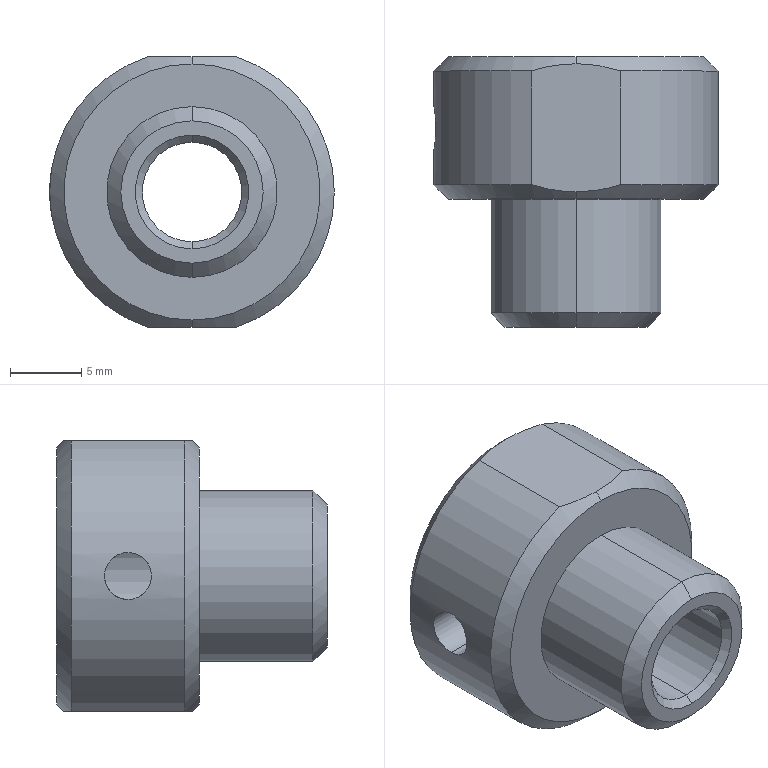Part | SolidWorks | features Chamfer 2, HoleWzd 2, ICE 1, Revolution 1 | 1 solid | 23 faces | box 20 x 19 x 19 mm | volume 3253 mm3 | cone 10 | cylinder 8 | plane 5 | commonest cylinder face diameters 3.3 x2 7 x2 12 x2 20 x2
STEP:
#1=CARTESIAN_POINT('',(-9.863,14.,-1.65));
#2=VERTEX_POINT('',#1);
#3=CARTESIAN_POINT('',(-9.863,14.,1.65));
#4=VERTEX_POINT('',#3);
#5=CARTESIAN_POINT('',(-9.863,14.,-1.65));
#6=CARTESIAN_POINT('',(-9.863,13.891,-1.65));
#7=CARTESIAN_POINT('',(-9.865,13.784,-1.639));
#8=CARTESIAN_POINT('',(-9.872,13.572,-1.597));
#9=CARTESIAN_POINT('',(-9.877,13.467,-1.565));
#10=CARTESIAN_POINT('',(-9.89,13.268,-1.483));
#11=CARTESIAN_POINT('',(-9.897,13.173,-1.432));
#12=CARTESIAN_POINT('',(-9.914,12.994,-1.312));
#13=CARTESIAN_POINT('',(-9.923,12.909,-1.243));
#14=CARTESIAN_POINT('',(-9.95,12.681,-1.015));
#15=CARTESIAN_POINT('',(-9.967,12.559,-0.8311));
#16=CARTESIAN_POINT('',(-9.993,12.394,-0.4342));
#17=CARTESIAN_POINT('',(-10.,12.35,-0.2172));
#18=CARTESIAN_POINT('',(-10.,12.35,0.1103));
#19=CARTESIAN_POINT('',(-9.998,12.361,0.2177));
#20=CARTESIAN_POINT('',(-9.991,12.403,0.4287));
#21=CARTESIAN_POINT('',(-9.986,12.435,0.5336));
#22=CARTESIAN_POINT('',(-9.974,12.518,0.7333));
#23=CARTESIAN_POINT('',(-9.966,12.569,0.8279));
#24=CARTESIAN_POINT('',(-9.95,12.689,1.007));
#25=CARTESIAN_POINT('',(-9.941,12.758,1.092));
#26=CARTESIAN_POINT('',(-9.914,12.986,1.319));
#27=CARTESIAN_POINT('',(-9.896,13.17,1.442));
#28=CARTESIAN_POINT('',(-9.87,13.567,1.607));
#29=CARTESIAN_POINT('',(-9.863,13.784,1.65));
#30=CARTESIAN_POINT('',(-9.863,14.,1.65));
#31=B_SPLINE_CURVE_WITH_KNOTS('',3,(#5,#6,#7,#8,#9,#10,#11,#12,#13,#14,#15,#16,#17,#18,#19,#20,#21,#22,#23,#24,#25,#26,#27,#28,#29,#30),.UNSPECIFIED.,.F.,.F.,(4,2,2,2,2,2,2,2,2,2,2,2,4),(0.007752,0.008074,0.008397,0.00872,0.009043,0.009689,0.01033,0.01066,0.01098,0.0113,0.01163,0.01227,0.01292),.UNSPECIFIED.);
#32=EDGE_CURVE('',#2,#4,#31,.T.);
#33=ORIENTED_EDGE('',*,*,#32,.T.);
#34=CARTESIAN_POINT('',(-3.087,14.,1.65));
#35=VERTEX_POINT('',#34);
#36=CARTESIAN_POINT('',(0.,14.,1.65));
#37=DIRECTION('',(1.,0.,0.));
#38=VECTOR('',#37,1000.);
#39=LINE('',#36,#38);
#40=EDGE_CURVE('',#4,#35,#39,.T.);
#41=ORIENTED_EDGE('',*,*,#40,.T.);
#42=CARTESIAN_POINT('',(-3.087,14.,-1.65));
#43=VERTEX_POINT('',#42);
#44=CARTESIAN_POINT('',(-3.087,14.,-1.65));
#45=CARTESIAN_POINT('',(-3.087,13.889,-1.65));
#46=CARTESIAN_POINT('',(-3.093,13.781,-1.639));
#47=CARTESIAN_POINT('',(-3.115,13.568,-1.596));
#48=CARTESIAN_POINT('',(-3.132,13.462,-1.564));
#49=CARTESIAN_POINT('',(-3.192,13.164,-1.439));
#50=CARTESIAN_POINT('',(-3.247,12.983,-1.317));
#51=CARTESIAN_POINT('',(-3.353,12.684,-1.017));
#52=CARTESIAN_POINT('',(-3.405,12.561,-0.836));
#53=CARTESIAN_POINT('',(-3.46,12.437,-0.5386));
#54=CARTESIAN_POINT('',(-3.475,12.404,-0.4329));
#55=CARTESIAN_POINT('',(-3.495,12.361,-0.2189));
#56=CARTESIAN_POINT('',(-3.5,12.35,-0.1106));
#57=CARTESIAN_POINT('',(-3.5,12.35,0.1086));
#58=CARTESIAN_POINT('',(-3.495,12.361,0.2196));
#59=CARTESIAN_POINT('',(-3.475,12.404,0.433));
#60=CARTESIAN_POINT('',(-3.46,12.436,0.5376));
#61=CARTESIAN_POINT('',(-3.423,12.52,0.7382));
#62=CARTESIAN_POINT('',(-3.401,12.571,0.8325));
#63=CARTESIAN_POINT('',(-3.352,12.691,1.01));
#64=CARTESIAN_POINT('',(-3.326,12.76,1.093));
#65=CARTESIAN_POINT('',(-3.246,12.985,1.318));
#66=CARTESIAN_POINT('',(-3.191,13.166,1.44));
#67=CARTESIAN_POINT('',(-3.112,13.562,1.605));
#68=CARTESIAN_POINT('',(-3.087,13.782,1.65));
#69=CARTESIAN_POINT('',(-3.087,14.,1.65));
#70=B_SPLINE_CURVE_WITH_KNOTS('',3,(#44,#45,#46,#47,#48,#49,#50,#51,#52,#53,#54,#55,#56,#57,#58,#59,#60,#61,#62,#63,#64,#65,#66,#67,#68,#69),.UNSPECIFIED.,.F.,.F.,(4,2,2,2,2,2,2,2,2,2,2,2,4),(0.,0.0003273,0.0006546,0.001309,0.001964,0.002291,0.002619,0.002946,0.003273,0.0036,0.003928,0.004582,0.005237),.UNSPECIFIED.);
#71=EDGE_CURVE('',#43,#35,#70,.T.);
#72=ORIENTED_EDGE('',*,*,#71,.F.);
#73=CARTESIAN_POINT('',(0.,14.,-1.65));
#74=DIRECTION('',(1.,0.,0.));
#75=VECTOR('',#74,1000.);
#76=LINE('',#73,#75);
#77=EDGE_CURVE('',#2,#43,#76,.T.);
#78=ORIENTED_EDGE('',*,*,#77,.F.);
#79=EDGE_LOOP('',(#33,#41,#72,#78));
#80=FACE_OUTER_BOUND('',#79,.T.);
#81=CARTESIAN_POINT('',(0.,14.,0.));
#82=DIRECTION('',(1.,0.,0.));
#83=DIRECTION('',(0.,0.,-1.));
#84=AXIS2_PLACEMENT_3D('',#81,#82,#83);
#85=CYLINDRICAL_SURFACE('',#84,1.65);
#86=ADVANCED_FACE('',(#80),#85,.F.);
#87=CARTESIAN_POINT('',(0.,18.5,-3.5));
#88=VERTEX_POINT('',#87);
#89=CARTESIAN_POINT('',(0.,18.5,3.5));
#90=VERTEX_POINT('',#89);
#91=CARTESIAN_POINT('',(0.,18.5,0.));
#92=DIRECTION('',(0.,1.,0.));
#93=DIRECTION('',(0.,0.,1.));
#94=AXIS2_PLACEMENT_3D('',#91,#92,#93);
#95=CIRCLE('',#94,3.5);
#96=EDGE_CURVE('',#88,#90,#95,.T.);
#97=ORIENTED_EDGE('',*,*,#96,.F.);
#98=CARTESIAN_POINT('',(0.,19.,-4.));
#99=VERTEX_POINT('',#98);
#100=CARTESIAN_POINT('',(0.,18.5,-3.5));
#101=DIRECTION('',(0.,0.7071,-0.7071));
#102=VECTOR('',#101,1000.);
#103=LINE('',#100,#102);
#104=EDGE_CURVE('',#88,#99,#103,.T.);
#105=ORIENTED_EDGE('',*,*,#104,.T.);
#106=CARTESIAN_POINT('',(0.,19.,4.));
#107=VERTEX_POINT('',#106);
#108=CARTESIAN_POINT('',(0.,19.,0.));
#109=DIRECTION('',(0.,-1.,0.));
#110=DIRECTION('',(0.,0.,1.));
#111=AXIS2_PLACEMENT_3D('',#108,#109,#110);
#112=CIRCLE('',#111,4.);
#113=EDGE_CURVE('',#107,#99,#112,.T.);
#114=ORIENTED_EDGE('',*,*,#113,.F.);
#115=CARTESIAN_POINT('',(0.,18.5,3.5));
#116=DIRECTION('',(0.,0.7071,0.7071));
#117=VECTOR('',#116,1000.);
#118=LINE('',#115,#117);
#119=EDGE_CURVE('',#90,#107,#118,.T.);
#120=ORIENTED_EDGE('',*,*,#119,.F.);
#121=EDGE_LOOP('',(#97,#105,#114,#120));
#122=FACE_OUTER_BOUND('',#121,.T.);
#123=CARTESIAN_POINT('',(0.,18.5,0.));
#124=DIRECTION('',(0.,1.,0.));
#125=DIRECTION('',(0.,0.,1.));
#126=AXIS2_PLACEMENT_3D('',#123,#124,#125);
#127=CONICAL_SURFACE('',#126,3.5,0.7854);
#128=ADVANCED_FACE('',(#122),#127,.F.);
#129=CARTESIAN_POINT('',(0.,0.5,3.5));
#130=VERTEX_POINT('',#129);
#131=CARTESIAN_POINT('',(0.,0.5,-3.5));
#132=VERTEX_POINT('',#131);
#133=CARTESIAN_POINT('',(0.,0.5,0.));
#134=DIRECTION('',(0.,-1.,0.));
#135=DIRECTION('',(0.,0.,-1.));
#136=AXIS2_PLACEMENT_3D('',#133,#134,#135);
#137=CIRCLE('',#136,3.5);
#138=EDGE_CURVE('',#130,#132,#137,.T.);
#139=ORIENTED_EDGE('',*,*,#138,.F.);
#140=CARTESIAN_POINT('',(0.,0.,4.));
#141=VERTEX_POINT('',#140);
#142=CARTESIAN_POINT('',(0.,0.,4.));
#143=DIRECTION('',(0.,-0.7071,0.7071));
#144=VECTOR('',#143,1000.);
#145=LINE('',#142,#144);
#146=EDGE_CURVE('',#130,#141,#145,.T.);
#147=ORIENTED_EDGE('',*,*,#146,.T.);
#148=CARTESIAN_POINT('',(0.,0.,-4.));
#149=VERTEX_POINT('',#148);
#150=CARTESIAN_POINT('',(0.,0.,0.));
#151=DIRECTION('',(0.,1.,0.));
#152=DIRECTION('',(0.,0.,-1.));
#153=AXIS2_PLACEMENT_3D('',#150,#151,#152);
#154=CIRCLE('',#153,4.);
#155=EDGE_CURVE('',#149,#141,#154,.T.);
#156=ORIENTED_EDGE('',*,*,#155,.F.);
#157=CARTESIAN_POINT('',(0.,0.,-4.));
#158=DIRECTION('',(0.,-0.7071,-0.7071));
#159=VECTOR('',#158,1000.);
#160=LINE('',#157,#159);
#161=EDGE_CURVE('',#132,#149,#160,.T.);
#162=ORIENTED_EDGE('',*,*,#161,.F.);
#163=EDGE_LOOP('',(#139,#147,#156,#162));
#164=FACE_OUTER_BOUND('',#163,.T.);
#165=CARTESIAN_POINT('',(0.,0.,0.));
#166=DIRECTION('',(0.,-1.,0.));
#167=DIRECTION('',(0.,0.,-1.));
#168=AXIS2_PLACEMENT_3D('',#165,#166,#167);
#169=CONICAL_SURFACE('',#168,4.,0.7854);
#170=ADVANCED_FACE('',(#164),#169,.F.);
#171=CARTESIAN_POINT('',(0.,0.,-5.));
#172=VERTEX_POINT('',#171);
#173=CARTESIAN_POINT('',(0.,0.,5.));
#174=VERTEX_POINT('',#173);
#175=CARTESIAN_POINT('',(0.,0.,0.));
#176=DIRECTION('',(0.,-1.,0.));
#177=DIRECTION('',(0.,0.,-1.));
#178=AXIS2_PLACEMENT_3D('',#175,#176,#177);
#179=CIRCLE('',#178,5.);
#180=EDGE_CURVE('',#172,#174,#179,.T.);
#181=ORIENTED_EDGE('',*,*,#180,.F.);
#182=CARTESIAN_POINT('',(0.,1.,-6.));
#183=VERTEX_POINT('',#182);
#184=CARTESIAN_POINT('',(0.,0.,-5.));
#185=DIRECTION('',(0.,0.7071,-0.7071));
#186=VECTOR('',#185,1000.);
#187=LINE('',#184,#186);
#188=EDGE_CURVE('',#172,#183,#187,.T.);
#189=ORIENTED_EDGE('',*,*,#188,.T.);
#190=CARTESIAN_POINT('',(0.,1.,6.));
#191=VERTEX_POINT('',#190);
#192=CARTESIAN_POINT('',(0.,1.,0.));
#193=DIRECTION('',(0.,1.,0.));
#194=DIRECTION('',(0.,0.,-1.));
#195=AXIS2_PLACEMENT_3D('',#192,#193,#194);
#196=CIRCLE('',#195,6.);
#197=EDGE_CURVE('',#191,#183,#196,.T.);
#198=ORIENTED_EDGE('',*,*,#197,.F.);
#199=CARTESIAN_POINT('',(0.,0.,5.));
#200=DIRECTION('',(0.,0.7071,0.7071));
#201=VECTOR('',#200,1000.);
#202=LINE('',#199,#201);
#203=EDGE_CURVE('',#174,#191,#202,.T.);
#204=ORIENTED_EDGE('',*,*,#203,.F.);
#205=EDGE_LOOP('',(#181,#189,#198,#204));
#206=FACE_OUTER_BOUND('',#205,.T.);
#207=CARTESIAN_POINT('',(0.,0.,0.));
#208=DIRECTION('',(0.,1.,0.));
#209=DIRECTION('',(0.,0.,1.));
#210=AXIS2_PLACEMENT_3D('',#207,#208,#209);
#211=CONICAL_SURFACE('',#210,5.,0.7854);
#212=ADVANCED_FACE('',(#206),#211,.T.);
#213=CARTESIAN_POINT('',(0.,9.,-9.));
#214=VERTEX_POINT('',#213);
#215=CARTESIAN_POINT('',(0.,9.,9.));
#216=VERTEX_POINT('',#215);
#217=CARTESIAN_POINT('',(0.,9.,0.));
#218=DIRECTION('',(0.,-1.,0.));
#219=DIRECTION('',(0.,0.,-1.));
#220=AXIS2_PLACEMENT_3D('',#217,#218,#219);
#221=CIRCLE('',#220,9.);
#222=EDGE_CURVE('',#214,#216,#221,.T.);
#223=ORIENTED_EDGE('',*,*,#222,.F.);
#224=CARTESIAN_POINT('',(0.,9.5,-9.5));
#225=VERTEX_POINT('',#224);
#226=CARTESIAN_POINT('',(0.,9.,-9.));
#227=DIRECTION('',(0.,0.7071,-0.7071));
#228=VECTOR('',#227,1000.);
#229=LINE('',#226,#228);
#230=EDGE_CURVE('',#214,#225,#229,.T.);
#231=ORIENTED_EDGE('',*,*,#230,.T.);
#232=CARTESIAN_POINT('',(3.122,10.,-9.5));
#233=VERTEX_POINT('',#232);
#234=CARTESIAN_POINT('',(3.122,10.,-9.5));
#235=CARTESIAN_POINT('',(2.615,9.841,-9.5));
#236=CARTESIAN_POINT('',(2.101,9.716,-9.5));
#237=CARTESIAN_POINT('',(1.321,9.588,-9.5));
#238=CARTESIAN_POINT('',(1.059,9.555,-9.5));
#239=CARTESIAN_POINT('',(0.5321,9.511,-9.5));
#240=CARTESIAN_POINT('',(0.2655,9.5,-9.5));
#241=CARTESIAN_POINT('',(0.,9.5,-9.5));
#242=B_SPLINE_CURVE_WITH_KNOTS('',3,(#234,#235,#236,#237,#238,#239,#240,#241),.UNSPECIFIED.,.F.,.F.,(4,2,2,4),(0.,0.001581,0.002372,0.003163),.UNSPECIFIED.);
#243=EDGE_CURVE('',#233,#225,#242,.T.);
#244=ORIENTED_EDGE('',*,*,#243,.F.);
#245=CARTESIAN_POINT('',(3.122,10.,9.5));
#246=VERTEX_POINT('',#245);
#247=CARTESIAN_POINT('',(0.,10.,0.));
#248=DIRECTION('',(0.,1.,0.));
#249=DIRECTION('',(0.,0.,1.));
#250=AXIS2_PLACEMENT_3D('',#247,#248,#249);
#251=CIRCLE('',#250,10.);
#252=EDGE_CURVE('',#246,#233,#251,.T.);
#253=ORIENTED_EDGE('',*,*,#252,.F.);
#254=CARTESIAN_POINT('',(0.,9.5,9.5));
#255=VERTEX_POINT('',#254);
#256=CARTESIAN_POINT('',(0.,9.5,9.5));
#257=CARTESIAN_POINT('',(1.067,9.5,9.5));
#258=CARTESIAN_POINT('',(2.106,9.682,9.5));
#259=CARTESIAN_POINT('',(3.122,10.,9.5));
#260=B_SPLINE_CURVE_WITH_KNOTS('',3,(#256,#257,#258,#259),.UNSPECIFIED.,.F.,.F.,(4,4),(0.003163,0.006342),.UNSPECIFIED.);
#261=EDGE_CURVE('',#255,#246,#260,.T.);
#262=ORIENTED_EDGE('',*,*,#261,.F.);
#263=CARTESIAN_POINT('',(0.,9.,9.));
#264=DIRECTION('',(0.,0.7071,0.7071));
#265=VECTOR('',#264,1000.);
#266=LINE('',#263,#265);
#267=EDGE_CURVE('',#216,#255,#266,.T.);
#268=ORIENTED_EDGE('',*,*,#267,.F.);
#269=EDGE_LOOP('',(#223,#231,#244,#253,#262,#268));
#270=FACE_OUTER_BOUND('',#269,.T.);
#271=CARTESIAN_POINT('',(0.,9.,0.));
#272=DIRECTION('',(0.,1.,0.));
#273=DIRECTION('',(0.,0.,1.));
#274=AXIS2_PLACEMENT_3D('',#271,#272,#273);
#275=CONICAL_SURFACE('',#274,9.,0.7854);
#276=ADVANCED_FACE('',(#270),#275,.T.);
#277=CARTESIAN_POINT('',(0.,19.,9.));
#278=VERTEX_POINT('',#277);
#279=CARTESIAN_POINT('',(0.,19.,-9.));
#280=VERTEX_POINT('',#279);
#281=CARTESIAN_POINT('',(0.,19.,0.));
#282=DIRECTION('',(0.,1.,0.));
#283=DIRECTION('',(0.,0.,1.));
#284=AXIS2_PLACEMENT_3D('',#281,#282,#283);
#285=CIRCLE('',#284,9.);
#286=EDGE_CURVE('',#278,#280,#285,.T.);
#287=ORIENTED_EDGE('',*,*,#286,.F.);
#288=CARTESIAN_POINT('',(0.,18.5,9.5));
#289=VERTEX_POINT('',#288);
#290=CARTESIAN_POINT('',(0.,18.,10.));
#291=DIRECTION('',(0.,-0.7071,0.7071));
#292=VECTOR('',#291,1000.);
#293=LINE('',#290,#292);
#294=EDGE_CURVE('',#278,#289,#293,.T.);
#295=ORIENTED_EDGE('',*,*,#294,.T.);
#296=CARTESIAN_POINT('',(3.122,18.,9.5));
#297=VERTEX_POINT('',#296);
#298=CARTESIAN_POINT('',(3.122,18.,9.5));
#299=CARTESIAN_POINT('',(2.615,18.159,9.5));
#300=CARTESIAN_POINT('',(2.101,18.284,9.5));
#301=CARTESIAN_POINT('',(1.321,18.412,9.5));
#302=CARTESIAN_POINT('',(1.059,18.445,9.5));
#303=CARTESIAN_POINT('',(0.5321,18.489,9.5));
#304=CARTESIAN_POINT('',(0.2655,18.5,9.5));
#305=CARTESIAN_POINT('',(0.,18.5,9.5));
#306=B_SPLINE_CURVE_WITH_KNOTS('',3,(#298,#299,#300,#301,#302,#303,#304,#305),.UNSPECIFIED.,.F.,.F.,(4,2,2,4),(0.,0.001581,0.002372,0.003163),.UNSPECIFIED.);
#307=EDGE_CURVE('',#297,#289,#306,.T.);
#308=ORIENTED_EDGE('',*,*,#307,.F.);
#309=CARTESIAN_POINT('',(3.122,18.,-9.5));
#310=VERTEX_POINT('',#309);
#311=CARTESIAN_POINT('',(0.,18.,0.));
#312=DIRECTION('',(0.,-1.,0.));
#313=DIRECTION('',(0.,0.,-1.));
#314=AXIS2_PLACEMENT_3D('',#311,#312,#313);
#315=CIRCLE('',#314,10.);
#316=EDGE_CURVE('',#310,#297,#315,.T.);
#317=ORIENTED_EDGE('',*,*,#316,.F.);
#318=CARTESIAN_POINT('',(0.,18.5,-9.5));
#319=VERTEX_POINT('',#318);
#320=CARTESIAN_POINT('',(0.,18.5,-9.5));
#321=CARTESIAN_POINT('',(1.067,18.5,-9.5));
#322=CARTESIAN_POINT('',(2.106,18.318,-9.5));
#323=CARTESIAN_POINT('',(3.122,18.,-9.5));
#324=B_SPLINE_CURVE_WITH_KNOTS('',3,(#320,#321,#322,#323),.UNSPECIFIED.,.F.,.F.,(4,4),(0.003163,0.006342),.UNSPECIFIED.);
#325=EDGE_CURVE('',#319,#310,#324,.T.);
#326=ORIENTED_EDGE('',*,*,#325,.F.);
#327=CARTESIAN_POINT('',(0.,18.,-10.));
#328=DIRECTION('',(0.,-0.7071,-0.7071));
#329=VECTOR('',#328,1000.);
#330=LINE('',#327,#329);
#331=EDGE_CURVE('',#280,#319,#330,.T.);
#332=ORIENTED_EDGE('',*,*,#331,.F.);
#333=EDGE_LOOP('',(#287,#295,#308,#317,#326,#332));
#334=FACE_OUTER_BOUND('',#333,.T.);
#335=CARTESIAN_POINT('',(0.,18.,0.));
#336=DIRECTION('',(0.,-1.,0.));
#337=DIRECTION('',(0.,0.,-1.));
#338=AXIS2_PLACEMENT_3D('',#335,#336,#337);
#339=CONICAL_SURFACE('',#338,10.,0.7854);
#340=ADVANCED_FACE('',(#334),#339,.T.);
#341=ORIENTED_EDGE('',*,*,#71,.T.);
#342=CARTESIAN_POINT('',(-3.087,14.,1.65));
#343=CARTESIAN_POINT('',(-3.087,14.109,1.65));
#344=CARTESIAN_POINT('',(-3.093,14.22,1.639));
#345=CARTESIAN_POINT('',(-3.115,14.434,1.596));
#346=CARTESIAN_POINT('',(-3.131,14.537,1.564));
#347=CARTESIAN_POINT('',(-3.192,14.837,1.438));
#348=CARTESIAN_POINT('',(-3.247,15.016,1.317));
#349=CARTESIAN_POINT('',(-3.326,15.242,1.091));
#350=CARTESIAN_POINT('',(-3.352,15.309,1.01));
#351=CARTESIAN_POINT('',(-3.401,15.429,0.8324));
#352=CARTESIAN_POINT('',(-3.423,15.481,0.7363));
#353=CARTESIAN_POINT('',(-3.46,15.564,0.5379));
#354=CARTESIAN_POINT('',(-3.475,15.595,0.4349));
#355=CARTESIAN_POINT('',(-3.495,15.639,0.2202));
#356=CARTESIAN_POINT('',(-3.5,15.65,0.11));
#357=CARTESIAN_POINT('',(-3.5,15.65,-0.217));
#358=CARTESIAN_POINT('',(-3.479,15.606,-0.4369));
#359=CARTESIAN_POINT('',(-3.423,15.481,-0.7362));
#360=CARTESIAN_POINT('',(-3.401,15.429,-0.8322));
#361=CARTESIAN_POINT('',(-3.353,15.31,-1.009));
#362=CARTESIAN_POINT('',(-3.326,15.242,-1.092));
#363=CARTESIAN_POINT('',(-3.273,15.09,-1.243));
#364=CARTESIAN_POINT('',(-3.246,15.008,-1.31));
#365=CARTESIAN_POINT('',(-3.196,14.832,-1.429));
#366=CARTESIAN_POINT('',(-3.172,14.736,-1.481));
#367=CARTESIAN_POINT('',(-3.132,14.537,-1.564));
#368=CARTESIAN_POINT('',(-3.115,14.435,-1.595));
#369=CARTESIAN_POINT('',(-3.093,14.222,-1.639));
#370=CARTESIAN_POINT('',(-3.087,14.111,-1.65));
#371=CARTESIAN_POINT('',(-3.087,14.,-1.65));
#372=B_SPLINE_CURVE_WITH_KNOTS('',3,(#342,#343,#344,#345,#346,#347,#348,#349,#350,#351,#352,#353,#354,#355,#356,#357,#358,#359,#360,#361,#362,#363,#364,#365,#366,#367,#368,#369,#370,#371),.UNSPECIFIED.,.F.,.F.,(4,2,2,2,2,2,2,2,2,2,2,2,2,2,4),(0.005237,0.005564,0.005891,0.006544,0.006871,0.007198,0.007525,0.007852,0.008506,0.008833,0.009159,0.009486,0.009813,0.01014,0.01047),.UNSPECIFIED.);
#373=EDGE_CURVE('',#35,#43,#372,.T.);
#374=ORIENTED_EDGE('',*,*,#373,.T.);
#375=EDGE_LOOP('',(#341,#374));
#376=FACE_BOUND('',#375,.T.);
#377=ORIENTED_EDGE('',*,*,#138,.T.);
#378=CARTESIAN_POINT('',(0.,19.,-3.5));
#379=DIRECTION('',(0.,1.,0.));
#380=VECTOR('',#379,1000.);
#381=LINE('',#378,#380);
#382=EDGE_CURVE('',#132,#88,#381,.T.);
#383=ORIENTED_EDGE('',*,*,#382,.T.);
#384=ORIENTED_EDGE('',*,*,#96,.T.);
#385=CARTESIAN_POINT('',(0.,19.,3.5));
#386=DIRECTION('',(0.,1.,0.));
#387=VECTOR('',#386,1000.);
#388=LINE('',#385,#387);
#389=EDGE_CURVE('',#130,#90,#388,.T.);
#390=ORIENTED_EDGE('',*,*,#389,.F.);
#391=EDGE_LOOP('',(#377,#383,#384,#390));
#392=FACE_OUTER_BOUND('',#391,.T.);
#393=CARTESIAN_POINT('',(0.,19.,0.));
#394=DIRECTION('',(0.,1.,0.));
#395=DIRECTION('',(0.,0.,1.));
#396=AXIS2_PLACEMENT_3D('',#393,#394,#395);
#397=CYLINDRICAL_SURFACE('',#396,3.5);
#398=ADVANCED_FACE('',(#376,#392),#397,.F.);
#399=CARTESIAN_POINT('',(0.,9.,-6.));
#400=VERTEX_POINT('',#399);
#401=CARTESIAN_POINT('',(0.,9.,6.));
#402=VERTEX_POINT('',#401);
#403=CARTESIAN_POINT('',(0.,9.,0.));
#404=DIRECTION('',(0.,-1.,0.));
#405=DIRECTION('',(0.,0.,-1.));
#406=AXIS2_PLACEMENT_3D('',#403,#404,#405);
#407=CIRCLE('',#406,6.);
#408=EDGE_CURVE('',#400,#402,#407,.T.);
#409=ORIENTED_EDGE('',*,*,#408,.T.);
#410=CARTESIAN_POINT('',(0.,0.,6.));
#411=DIRECTION('',(0.,-1.,0.));
#412=VECTOR('',#411,1000.);
#413=LINE('',#410,#412);
#414=EDGE_CURVE('',#402,#191,#413,.T.);
#415=ORIENTED_EDGE('',*,*,#414,.T.);
#416=ORIENTED_EDGE('',*,*,#197,.T.);
#417=CARTESIAN_POINT('',(0.,0.,-6.));
#418=DIRECTION('',(0.,-1.,0.));
#419=VECTOR('',#418,1000.);
#420=LINE('',#417,#419);
#421=EDGE_CURVE('',#400,#183,#420,.T.);
#422=ORIENTED_EDGE('',*,*,#421,.F.);
#423=EDGE_LOOP('',(#409,#415,#416,#422));
#424=FACE_OUTER_BOUND('',#423,.T.);
#425=CARTESIAN_POINT('',(0.,0.,0.));
#426=DIRECTION('',(0.,-1.,0.));
#427=DIRECTION('',(0.,0.,-1.));
#428=AXIS2_PLACEMENT_3D('',#425,#426,#427);
#429=CYLINDRICAL_SURFACE('',#428,6.);
#430=ADVANCED_FACE('',(#424),#429,.T.);
#431=CARTESIAN_POINT('',(0.,9.,0.));
#432=DIRECTION('',(0.,-1.,0.));
#433=DIRECTION('',(0.,0.,-1.));
#434=AXIS2_PLACEMENT_3D('',#431,#432,#433);
#435=CIRCLE('',#434,9.);
#436=EDGE_CURVE('',#216,#214,#435,.T.);
#437=ORIENTED_EDGE('',*,*,#436,.T.);
#438=ORIENTED_EDGE('',*,*,#222,.T.);
#439=EDGE_LOOP('',(#437,#438));
#440=FACE_OUTER_BOUND('',#439,.T.);
#441=ORIENTED_EDGE('',*,*,#408,.F.);
#442=CARTESIAN_POINT('',(0.,9.,0.));
#443=DIRECTION('',(0.,-1.,0.));
#444=DIRECTION('',(0.,0.,-1.));
#445=AXIS2_PLACEMENT_3D('',#442,#443,#444);
#446=CIRCLE('',#445,6.);
#447=EDGE_CURVE('',#402,#400,#446,.T.);
#448=ORIENTED_EDGE('',*,*,#447,.F.);
#449=EDGE_LOOP('',(#441,#448));
#450=FACE_BOUND('',#449,.T.);
#451=CARTESIAN_POINT('',(0.,9.,0.));
#452=DIRECTION('',(0.,-1.,0.));
#453=DIRECTION('',(0.,0.,-1.));
#454=AXIS2_PLACEMENT_3D('',#451,#452,#453);
#455=PLANE('',#454);
#456=ADVANCED_FACE('',(#440,#450),#455,.T.);
#457=CARTESIAN_POINT('',(3.122,0.,-9.5));
#458=DIRECTION('',(0.,1.,0.));
#459=VECTOR('',#458,1000.);
#460=LINE('',#457,#459);
#461=EDGE_CURVE('',#233,#310,#460,.T.);
#462=ORIENTED_EDGE('',*,*,#461,.T.);
#463=ORIENTED_EDGE('',*,*,#316,.T.);
#464=CARTESIAN_POINT('',(3.122,0.,9.5));
#465=DIRECTION('',(0.,-1.,0.));
#466=VECTOR('',#465,1000.);
#467=LINE('',#464,#466);
#468=EDGE_CURVE('',#297,#246,#467,.T.);
#469=ORIENTED_EDGE('',*,*,#468,.T.);
#470=ORIENTED_EDGE('',*,*,#252,.T.);
#471=EDGE_LOOP('',(#462,#463,#469,#470));
#472=FACE_OUTER_BOUND('',#471,.T.);
#473=CARTESIAN_POINT('',(0.,0.,0.));
#474=DIRECTION('',(0.,-1.,0.));
#475=DIRECTION('',(0.,0.,-1.));
#476=AXIS2_PLACEMENT_3D('',#473,#474,#475);
#477=CYLINDRICAL_SURFACE('',#476,10.);
#478=ADVANCED_FACE('',(#472),#477,.T.);
#479=ORIENTED_EDGE('',*,*,#32,.F.);
#480=CARTESIAN_POINT('',(-9.863,14.,1.65));
#481=CARTESIAN_POINT('',(-9.863,14.108,1.65));
#482=CARTESIAN_POINT('',(-9.865,14.217,1.639));
#483=CARTESIAN_POINT('',(-9.872,14.429,1.597));
#484=CARTESIAN_POINT('',(-9.877,14.532,1.566));
#485=CARTESIAN_POINT('',(-9.896,14.832,1.441));
#486=CARTESIAN_POINT('',(-9.914,15.014,1.32));
#487=CARTESIAN_POINT('',(-9.941,15.244,1.089));
#488=CARTESIAN_POINT('',(-9.95,15.312,1.006));
#489=CARTESIAN_POINT('',(-9.966,15.431,0.8278));
#490=CARTESIAN_POINT('',(-9.974,15.483,0.7312));
#491=CARTESIAN_POINT('',(-9.986,15.566,0.5315));
#492=CARTESIAN_POINT('',(-9.991,15.597,0.4286));
#493=CARTESIAN_POINT('',(-9.998,15.639,0.2168));
#494=CARTESIAN_POINT('',(-10.,15.65,0.1073));
#495=CARTESIAN_POINT('',(-10.,15.65,-0.216));
#496=CARTESIAN_POINT('',(-9.993,15.606,-0.4335));
#497=CARTESIAN_POINT('',(-9.967,15.442,-0.8307));
#498=CARTESIAN_POINT('',(-9.95,15.319,-1.014));
#499=CARTESIAN_POINT('',(-9.923,15.091,-1.243));
#500=CARTESIAN_POINT('',(-9.914,15.006,-1.312));
#501=CARTESIAN_POINT('',(-9.897,14.827,-1.432));
#502=CARTESIAN_POINT('',(-9.89,14.732,-1.482));
#503=CARTESIAN_POINT('',(-9.87,14.432,-1.607));
#504=CARTESIAN_POINT('',(-9.863,14.218,-1.65));
#505=CARTESIAN_POINT('',(-9.863,14.,-1.65));
#506=B_SPLINE_CURVE_WITH_KNOTS('',3,(#480,#481,#482,#483,#484,#485,#486,#487,#488,#489,#490,#491,#492,#493,#494,#495,#496,#497,#498,#499,#500,#501,#502,#503,#504,#505),.UNSPECIFIED.,.F.,.F.,(4,2,2,2,2,2,2,2,2,2,2,2,4),(0.002584,0.002907,0.00323,0.003876,0.004199,0.004522,0.004845,0.005168,0.005814,0.00646,0.006783,0.007106,0.007752),.UNSPECIFIED.);
#507=EDGE_CURVE('',#4,#2,#506,.T.);
#508=ORIENTED_EDGE('',*,*,#507,.F.);
#509=EDGE_LOOP('',(#479,#508));
#510=FACE_BOUND('',#509,.T.);
#511=CARTESIAN_POINT('',(-3.122,10.,9.5));
#512=VERTEX_POINT('',#511);
#513=CARTESIAN_POINT('',(-3.122,18.,9.5));
#514=VERTEX_POINT('',#513);
#515=CARTESIAN_POINT('',(-3.122,0.,9.5));
#516=DIRECTION('',(0.,1.,0.));
#517=VECTOR('',#516,1000.);
#518=LINE('',#515,#517);
#519=EDGE_CURVE('',#512,#514,#518,.T.);
#520=ORIENTED_EDGE('',*,*,#519,.T.);
#521=CARTESIAN_POINT('',(-3.122,18.,-9.5));
#522=VERTEX_POINT('',#521);
#523=CARTESIAN_POINT('',(0.,18.,0.));
#524=DIRECTION('',(0.,-1.,0.));
#525=DIRECTION('',(0.,0.,1.));
#526=AXIS2_PLACEMENT_3D('',#523,#524,#525);
#527=CIRCLE('',#526,10.);
#528=EDGE_CURVE('',#514,#522,#527,.T.);
#529=ORIENTED_EDGE('',*,*,#528,.T.);
#530=CARTESIAN_POINT('',(-3.122,10.,-9.5));
#531=VERTEX_POINT('',#530);
#532=CARTESIAN_POINT('',(-3.122,0.,-9.5));
#533=DIRECTION('',(0.,-1.,0.));
#534=VECTOR('',#533,1000.);
#535=LINE('',#532,#534);
#536=EDGE_CURVE('',#522,#531,#535,.T.);
#537=ORIENTED_EDGE('',*,*,#536,.T.);
#538=CARTESIAN_POINT('',(0.,10.,0.));
#539=DIRECTION('',(0.,1.,0.));
#540=DIRECTION('',(0.,0.,-1.));
#541=AXIS2_PLACEMENT_3D('',#538,#539,#540);
#542=CIRCLE('',#541,10.);
#543=EDGE_CURVE('',#531,#512,#542,.T.);
#544=ORIENTED_EDGE('',*,*,#543,.T.);
#545=EDGE_LOOP('',(#520,#529,#537,#544));
#546=FACE_OUTER_BOUND('',#545,.T.);
#547=CARTESIAN_POINT('',(0.,0.,0.));
#548=DIRECTION('',(0.,-1.,0.));
#549=DIRECTION('',(0.,0.,-1.));
#550=AXIS2_PLACEMENT_3D('',#547,#548,#549);
#551=CYLINDRICAL_SURFACE('',#550,10.);
#552=ADVANCED_FACE('',(#510,#546),#551,.T.);
#553=ORIENTED_EDGE('',*,*,#113,.T.);
#554=CARTESIAN_POINT('',(0.,19.,0.));
#555=DIRECTION('',(0.,-1.,0.));
#556=DIRECTION('',(0.,0.,1.));
#557=AXIS2_PLACEMENT_3D('',#554,#555,#556);
#558=CIRCLE('',#557,4.);
#559=EDGE_CURVE('',#99,#107,#558,.T.);
#560=ORIENTED_EDGE('',*,*,#559,.T.);
#561=EDGE_LOOP('',(#553,#560));
#562=FACE_BOUND('',#561,.T.);
#563=CARTESIAN_POINT('',(0.,19.,0.));
#564=DIRECTION('',(0.,1.,0.));
#565=DIRECTION('',(0.,0.,1.));
#566=AXIS2_PLACEMENT_3D('',#563,#564,#565);
#567=CIRCLE('',#566,9.);
#568=EDGE_CURVE('',#280,#278,#567,.T.);
#569=ORIENTED_EDGE('',*,*,#568,.T.);
#570=ORIENTED_EDGE('',*,*,#286,.T.);
#571=EDGE_LOOP('',(#569,#570));
#572=FACE_OUTER_BOUND('',#571,.T.);
#573=CARTESIAN_POINT('',(0.,19.,0.));
#574=DIRECTION('',(0.,1.,0.));
#575=DIRECTION('',(0.,0.,1.));
#576=AXIS2_PLACEMENT_3D('',#573,#574,#575);
#577=PLANE('',#576);
#578=ADVANCED_FACE('',(#562,#572),#577,.T.);
#579=ORIENTED_EDGE('',*,*,#155,.T.);
#580=CARTESIAN_POINT('',(0.,0.,0.));
#581=DIRECTION('',(0.,1.,0.));
#582=DIRECTION('',(0.,0.,-1.));
#583=AXIS2_PLACEMENT_3D('',#580,#581,#582);
#584=CIRCLE('',#583,4.);
#585=EDGE_CURVE('',#141,#149,#584,.T.);
#586=ORIENTED_EDGE('',*,*,#585,.T.);
#587=EDGE_LOOP('',(#579,#586));
#588=FACE_BOUND('',#587,.T.);
#589=CARTESIAN_POINT('',(0.,0.,0.));
#590=DIRECTION('',(0.,-1.,0.));
#591=DIRECTION('',(0.,0.,-1.));
#592=AXIS2_PLACEMENT_3D('',#589,#590,#591);
#593=CIRCLE('',#592,5.);
#594=EDGE_CURVE('',#174,#172,#593,.T.);
#595=ORIENTED_EDGE('',*,*,#594,.T.);
#596=ORIENTED_EDGE('',*,*,#180,.T.);
#597=EDGE_LOOP('',(#595,#596));
#598=FACE_OUTER_BOUND('',#597,.T.);
#599=CARTESIAN_POINT('',(0.,0.,0.));
#600=DIRECTION('',(0.,-1.,0.));
#601=DIRECTION('',(0.,0.,-1.));
#602=AXIS2_PLACEMENT_3D('',#599,#600,#601);
#603=PLANE('',#602);
#604=ADVANCED_FACE('',(#588,#598),#603,.T.);
#605=ORIENTED_EDGE('',*,*,#414,.F.);
#606=ORIENTED_EDGE('',*,*,#447,.T.);
#607=ORIENTED_EDGE('',*,*,#421,.T.);
#608=CARTESIAN_POINT('',(0.,1.,0.));
#609=DIRECTION('',(0.,1.,0.));
#610=DIRECTION('',(0.,0.,-1.));
#611=AXIS2_PLACEMENT_3D('',#608,#609,#610);
#612=CIRCLE('',#611,6.);
#613=EDGE_CURVE('',#183,#191,#612,.T.);
#614=ORIENTED_EDGE('',*,*,#613,.T.);
#615=EDGE_LOOP('',(#605,#606,#607,#614));
#616=FACE_OUTER_BOUND('',#615,.T.);
#617=CARTESIAN_POINT('',(0.,0.,0.));
#618=DIRECTION('',(0.,-1.,0.));
#619=DIRECTION('',(0.,0.,-1.));
#620=AXIS2_PLACEMENT_3D('',#617,#618,#619);
#621=CYLINDRICAL_SURFACE('',#620,6.);
#622=ADVANCED_FACE('',(#616),#621,.T.);
#623=ORIENTED_EDGE('',*,*,#382,.F.);
#624=CARTESIAN_POINT('',(0.,0.5,0.));
#625=DIRECTION('',(0.,-1.,0.));
#626=DIRECTION('',(0.,0.,-1.));
#627=AXIS2_PLACEMENT_3D('',#624,#625,#626);
#628=CIRCLE('',#627,3.5);
#629=EDGE_CURVE('',#132,#130,#628,.T.);
#630=ORIENTED_EDGE('',*,*,#629,.T.);
#631=ORIENTED_EDGE('',*,*,#389,.T.);
#632=CARTESIAN_POINT('',(0.,18.5,0.));
#633=DIRECTION('',(0.,1.,0.));
#634=DIRECTION('',(0.,0.,1.));
#635=AXIS2_PLACEMENT_3D('',#632,#633,#634);
#636=CIRCLE('',#635,3.5);
#637=EDGE_CURVE('',#90,#88,#636,.T.);
#638=ORIENTED_EDGE('',*,*,#637,.T.);
#639=EDGE_LOOP('',(#623,#630,#631,#638));
#640=FACE_OUTER_BOUND('',#639,.T.);
#641=CARTESIAN_POINT('',(0.,19.,0.));
#642=DIRECTION('',(0.,1.,0.));
#643=DIRECTION('',(0.,0.,1.));
#644=AXIS2_PLACEMENT_3D('',#641,#642,#643);
#645=CYLINDRICAL_SURFACE('',#644,3.5);
#646=ADVANCED_FACE('',(#640),#645,.F.);
#647=ORIENTED_EDGE('',*,*,#468,.F.);
#648=ORIENTED_EDGE('',*,*,#307,.T.);
#649=CARTESIAN_POINT('',(0.,18.5,9.5));
#650=CARTESIAN_POINT('',(-1.067,18.5,9.5));
#651=CARTESIAN_POINT('',(-2.106,18.318,9.5));
#652=CARTESIAN_POINT('',(-3.122,18.,9.5));
#653=B_SPLINE_CURVE_WITH_KNOTS('',3,(#649,#650,#651,#652),.UNSPECIFIED.,.F.,.F.,(4,4),(0.003163,0.006342),.UNSPECIFIED.);
#654=EDGE_CURVE('',#289,#514,#653,.T.);
#655=ORIENTED_EDGE('',*,*,#654,.T.);
#656=ORIENTED_EDGE('',*,*,#519,.F.);
#657=CARTESIAN_POINT('',(-3.122,10.,9.5));
#658=CARTESIAN_POINT('',(-2.615,9.841,9.5));
#659=CARTESIAN_POINT('',(-2.101,9.716,9.5));
#660=CARTESIAN_POINT('',(-1.321,9.588,9.5));
#661=CARTESIAN_POINT('',(-1.059,9.555,9.5));
#662=CARTESIAN_POINT('',(-0.5321,9.511,9.5));
#663=CARTESIAN_POINT('',(-0.2655,9.5,9.5));
#664=CARTESIAN_POINT('',(0.,9.5,9.5));
#665=B_SPLINE_CURVE_WITH_KNOTS('',3,(#657,#658,#659,#660,#661,#662,#663,#664),.UNSPECIFIED.,.F.,.F.,(4,2,2,4),(0.,0.001581,0.002372,0.003163),.UNSPECIFIED.);
#666=EDGE_CURVE('',#512,#255,#665,.T.);
#667=ORIENTED_EDGE('',*,*,#666,.T.);
#668=ORIENTED_EDGE('',*,*,#261,.T.);
#669=EDGE_LOOP('',(#647,#648,#655,#656,#667,#668));
#670=FACE_OUTER_BOUND('',#669,.T.);
#671=CARTESIAN_POINT('',(14.978,0.,9.5));
#672=DIRECTION('',(0.,0.,1.));
#673=DIRECTION('',(1.,0.,0.));
#674=AXIS2_PLACEMENT_3D('',#671,#672,#673);
#675=PLANE('',#674);
#676=ADVANCED_FACE('',(#670),#675,.T.);
#677=ORIENTED_EDGE('',*,*,#536,.F.);
#678=CARTESIAN_POINT('',(-3.122,18.,-9.5));
#679=CARTESIAN_POINT('',(-2.615,18.159,-9.5));
#680=CARTESIAN_POINT('',(-2.101,18.284,-9.5));
#681=CARTESIAN_POINT('',(-1.321,18.412,-9.5));
#682=CARTESIAN_POINT('',(-1.059,18.445,-9.5));
#683=CARTESIAN_POINT('',(-0.5321,18.489,-9.5));
#684=CARTESIAN_POINT('',(-0.2655,18.5,-9.5));
#685=CARTESIAN_POINT('',(0.,18.5,-9.5));
#686=B_SPLINE_CURVE_WITH_KNOTS('',3,(#678,#679,#680,#681,#682,#683,#684,#685),.UNSPECIFIED.,.F.,.F.,(4,2,2,4),(0.,0.001581,0.002372,0.003163),.UNSPECIFIED.);
#687=EDGE_CURVE('',#522,#319,#686,.T.);
#688=ORIENTED_EDGE('',*,*,#687,.T.);
#689=ORIENTED_EDGE('',*,*,#325,.T.);
#690=ORIENTED_EDGE('',*,*,#461,.F.);
#691=ORIENTED_EDGE('',*,*,#243,.T.);
#692=CARTESIAN_POINT('',(0.,9.5,-9.5));
#693=CARTESIAN_POINT('',(-1.067,9.5,-9.5));
#694=CARTESIAN_POINT('',(-2.106,9.682,-9.5));
#695=CARTESIAN_POINT('',(-3.122,10.,-9.5));
#696=B_SPLINE_CURVE_WITH_KNOTS('',3,(#692,#693,#694,#695),.UNSPECIFIED.,.F.,.F.,(4,4),(0.003163,0.006342),.UNSPECIFIED.);
#697=EDGE_CURVE('',#225,#531,#696,.T.);
#698=ORIENTED_EDGE('',*,*,#697,.T.);
#699=EDGE_LOOP('',(#677,#688,#689,#690,#691,#698));
#700=FACE_OUTER_BOUND('',#699,.T.);
#701=CARTESIAN_POINT('',(14.978,0.,-9.5));
#702=DIRECTION('',(0.,0.,-1.));
#703=DIRECTION('',(-1.,0.,0.));
#704=AXIS2_PLACEMENT_3D('',#701,#702,#703);
#705=PLANE('',#704);
#706=ADVANCED_FACE('',(#700),#705,.T.);
#707=ORIENTED_EDGE('',*,*,#294,.F.);
#708=ORIENTED_EDGE('',*,*,#568,.F.);
#709=ORIENTED_EDGE('',*,*,#331,.T.);
#710=ORIENTED_EDGE('',*,*,#687,.F.);
#711=ORIENTED_EDGE('',*,*,#528,.F.);
#712=ORIENTED_EDGE('',*,*,#654,.F.);
#713=EDGE_LOOP('',(#707,#708,#709,#710,#711,#712));
#714=FACE_OUTER_BOUND('',#713,.T.);
#715=CARTESIAN_POINT('',(0.,18.,0.));
#716=DIRECTION('',(0.,-1.,0.));
#717=DIRECTION('',(0.,0.,-1.));
#718=AXIS2_PLACEMENT_3D('',#715,#716,#717);
#719=CONICAL_SURFACE('',#718,10.,0.7854);
#720=ADVANCED_FACE('',(#714),#719,.T.);
#721=ORIENTED_EDGE('',*,*,#230,.F.);
#722=ORIENTED_EDGE('',*,*,#436,.F.);
#723=ORIENTED_EDGE('',*,*,#267,.T.);
#724=ORIENTED_EDGE('',*,*,#666,.F.);
#725=ORIENTED_EDGE('',*,*,#543,.F.);
#726=ORIENTED_EDGE('',*,*,#697,.F.);
#727=EDGE_LOOP('',(#721,#722,#723,#724,#725,#726));
#728=FACE_OUTER_BOUND('',#727,.T.);
#729=CARTESIAN_POINT('',(0.,9.,0.));
#730=DIRECTION('',(0.,1.,0.));
#731=DIRECTION('',(0.,0.,1.));
#732=AXIS2_PLACEMENT_3D('',#729,#730,#731);
#733=CONICAL_SURFACE('',#732,9.,0.7854);
#734=ADVANCED_FACE('',(#728),#733,.T.);
#735=ORIENTED_EDGE('',*,*,#188,.F.);
#736=ORIENTED_EDGE('',*,*,#594,.F.);
#737=ORIENTED_EDGE('',*,*,#203,.T.);
#738=ORIENTED_EDGE('',*,*,#613,.F.);
#739=EDGE_LOOP('',(#735,#736,#737,#738));
#740=FACE_OUTER_BOUND('',#739,.T.);
#741=CARTESIAN_POINT('',(0.,0.,0.));
#742=DIRECTION('',(0.,1.,0.));
#743=DIRECTION('',(0.,0.,1.));
#744=AXIS2_PLACEMENT_3D('',#741,#742,#743);
#745=CONICAL_SURFACE('',#744,5.,0.7854);
#746=ADVANCED_FACE('',(#740),#745,.T.);
#747=ORIENTED_EDGE('',*,*,#146,.F.);
#748=ORIENTED_EDGE('',*,*,#629,.F.);
#749=ORIENTED_EDGE('',*,*,#161,.T.);
#750=ORIENTED_EDGE('',*,*,#585,.F.);
#751=EDGE_LOOP('',(#747,#748,#749,#750));
#752=FACE_OUTER_BOUND('',#751,.T.);
#753=CARTESIAN_POINT('',(0.,0.,0.));
#754=DIRECTION('',(0.,-1.,0.));
#755=DIRECTION('',(0.,0.,-1.));
#756=AXIS2_PLACEMENT_3D('',#753,#754,#755);
#757=CONICAL_SURFACE('',#756,4.,0.7854);
#758=ADVANCED_FACE('',(#752),#757,.F.);
#759=ORIENTED_EDGE('',*,*,#104,.F.);
#760=ORIENTED_EDGE('',*,*,#637,.F.);
#761=ORIENTED_EDGE('',*,*,#119,.T.);
#762=ORIENTED_EDGE('',*,*,#559,.F.);
#763=EDGE_LOOP('',(#759,#760,#761,#762));
#764=FACE_OUTER_BOUND('',#763,.T.);
#765=CARTESIAN_POINT('',(0.,18.5,0.));
#766=DIRECTION('',(0.,1.,0.));
#767=DIRECTION('',(0.,0.,1.));
#768=AXIS2_PLACEMENT_3D('',#765,#766,#767);
#769=CONICAL_SURFACE('',#768,3.5,0.7854);
#770=ADVANCED_FACE('',(#764),#769,.F.);
#771=ORIENTED_EDGE('',*,*,#40,.F.);
#772=ORIENTED_EDGE('',*,*,#507,.T.);
#773=ORIENTED_EDGE('',*,*,#77,.T.);
#774=ORIENTED_EDGE('',*,*,#373,.F.);
#775=EDGE_LOOP('',(#771,#772,#773,#774));
#776=FACE_OUTER_BOUND('',#775,.T.);
#777=CARTESIAN_POINT('',(0.,14.,0.));
#778=DIRECTION('',(1.,0.,0.));
#779=DIRECTION('',(0.,0.,-1.));
#780=AXIS2_PLACEMENT_3D('',#777,#778,#779);
#781=CYLINDRICAL_SURFACE('',#780,1.65);
#782=ADVANCED_FACE('',(#776),#781,.F.);
#783=CLOSED_SHELL('',(#86,#128,#170,#212,#276,#340,#398,#430,#456,#478,#552,#578,#604,#622,#646,#676,#706,#720,#734,#746,#758,#770,#782));
#784=MANIFOLD_SOLID_BREP('',#783);
#785=CARTESIAN_POINT('',(0.,0.,0.));
#786=DIRECTION('',(0.,0.,1.));
#787=DIRECTION('',(1.,0.,0.));
#788=AXIS2_PLACEMENT_3D('',#785,#786,#787);
#789=(LENGTH_UNIT()NAMED_UNIT(*)SI_UNIT(.MILLI.,.METRE.));
#790=UNCERTAINTY_MEASURE_WITH_UNIT(LENGTH_MEASURE(0.00001),#789,'','');
#791=(NAMED_UNIT(*)PLANE_ANGLE_UNIT()SI_UNIT($,.RADIAN.));
#792=(NAMED_UNIT(*)SI_UNIT($,.STERADIAN.)SOLID_ANGLE_UNIT());
#793=(GEOMETRIC_REPRESENTATION_CONTEXT(3)GLOBAL_UNCERTAINTY_ASSIGNED_CONTEXT((#790))GLOBAL_UNIT_ASSIGNED_CONTEXT((#789,#791,#792))REPRESENTATION_CONTEXT('',''));
#794=ADVANCED_BREP_SHAPE_REPRESENTATION('',(#784,#788),#793);